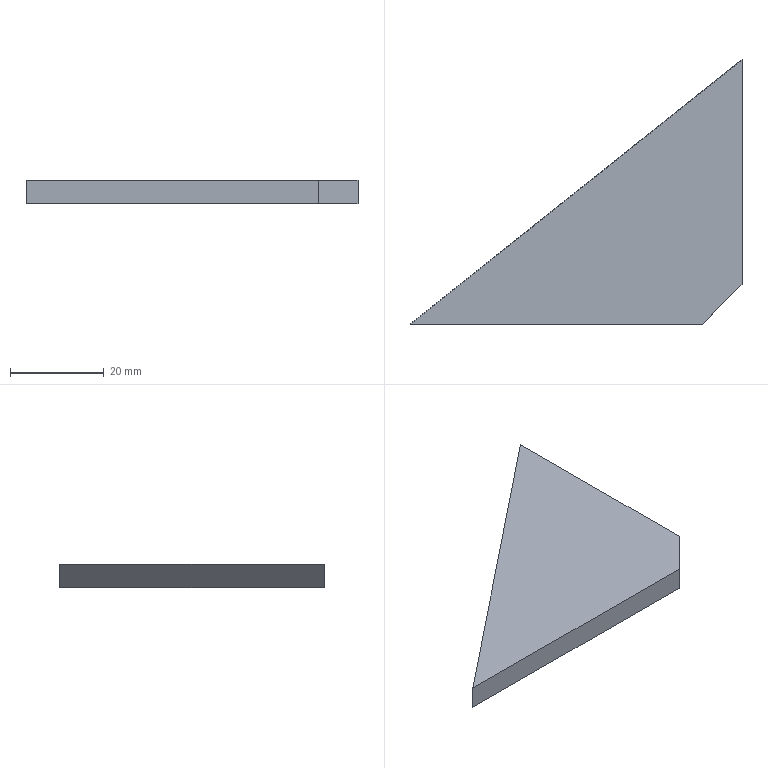Part | SolidWorks | features Extrusion 1, ICE 1 | 1 solid | 6 faces | box 70.878 x 56.464 x 5 mm | volume 9823 mm3 | plane 6
STEP:
#1=CARTESIAN_POINT('',(-5.,0.,0.));
#2=VERTEX_POINT('',#1);
#3=CARTESIAN_POINT('',(-75.878,-56.464,0.));
#4=VERTEX_POINT('',#3);
#5=CARTESIAN_POINT('',(-113.536,-86.464,0.));
#6=DIRECTION('',(-0.7821,-0.6231,0.));
#7=VECTOR('',#6,1000.);
#8=LINE('',#5,#7);
#9=EDGE_CURVE('',#2,#4,#8,.T.);
#10=ORIENTED_EDGE('',*,*,#9,.T.);
#11=CARTESIAN_POINT('',(-75.878,-56.464,5.));
#12=VERTEX_POINT('',#11);
#13=CARTESIAN_POINT('',(-75.878,-56.464,5.));
#14=DIRECTION('',(0.,0.,1.));
#15=VECTOR('',#14,1000.);
#16=LINE('',#13,#15);
#17=EDGE_CURVE('',#4,#12,#16,.T.);
#18=ORIENTED_EDGE('',*,*,#17,.T.);
#19=CARTESIAN_POINT('',(-5.,0.,5.));
#20=VERTEX_POINT('',#19);
#21=CARTESIAN_POINT('',(-113.536,-86.464,5.));
#22=DIRECTION('',(-0.7821,-0.6231,0.));
#23=VECTOR('',#22,1000.);
#24=LINE('',#21,#23);
#25=EDGE_CURVE('',#20,#12,#24,.T.);
#26=ORIENTED_EDGE('',*,*,#25,.F.);
#27=CARTESIAN_POINT('',(-5.,0.,5.));
#28=DIRECTION('',(0.,0.,-1.));
#29=VECTOR('',#28,1000.);
#30=LINE('',#27,#29);
#31=EDGE_CURVE('',#20,#2,#30,.T.);
#32=ORIENTED_EDGE('',*,*,#31,.T.);
#33=EDGE_LOOP('',(#10,#18,#26,#32));
#34=FACE_OUTER_BOUND('',#33,.T.);
#35=CARTESIAN_POINT('',(-113.536,-86.464,5.));
#36=DIRECTION('',(0.6231,-0.7821,0.));
#37=DIRECTION('',(0.7821,0.6231,0.));
#38=AXIS2_PLACEMENT_3D('',#35,#36,#37);
#39=PLANE('',#38);
#40=ADVANCED_FACE('',(#34),#39,.F.);
#41=CARTESIAN_POINT('',(-13.536,-56.464,5.));
#42=VERTEX_POINT('',#41);
#43=CARTESIAN_POINT('',(-5.,-47.929,5.));
#44=VERTEX_POINT('',#43);
#45=CARTESIAN_POINT('',(-5.,-47.929,5.));
#46=DIRECTION('',(0.7071,0.7071,0.));
#47=VECTOR('',#46,1000.);
#48=LINE('',#45,#47);
#49=EDGE_CURVE('',#42,#44,#48,.T.);
#50=ORIENTED_EDGE('',*,*,#49,.F.);
#51=CARTESIAN_POINT('',(-13.536,-56.464,0.));
#52=VERTEX_POINT('',#51);
#53=CARTESIAN_POINT('',(-13.536,-56.464,-355.));
#54=DIRECTION('',(0.,0.,1.));
#55=VECTOR('',#54,1000.);
#56=LINE('',#53,#55);
#57=EDGE_CURVE('',#52,#42,#56,.T.);
#58=ORIENTED_EDGE('',*,*,#57,.F.);
#59=CARTESIAN_POINT('',(-5.,-47.929,0.));
#60=VERTEX_POINT('',#59);
#61=CARTESIAN_POINT('',(-5.,-47.929,0.));
#62=DIRECTION('',(0.7071,0.7071,0.));
#63=VECTOR('',#62,1000.);
#64=LINE('',#61,#63);
#65=EDGE_CURVE('',#52,#60,#64,.T.);
#66=ORIENTED_EDGE('',*,*,#65,.T.);
#67=CARTESIAN_POINT('',(-5.,-47.929,5.));
#68=DIRECTION('',(0.,0.,-1.));
#69=VECTOR('',#68,1000.);
#70=LINE('',#67,#69);
#71=EDGE_CURVE('',#44,#60,#70,.T.);
#72=ORIENTED_EDGE('',*,*,#71,.F.);
#73=EDGE_LOOP('',(#50,#58,#66,#72));
#74=FACE_OUTER_BOUND('',#73,.T.);
#75=CARTESIAN_POINT('',(-5.,-47.929,5.));
#76=DIRECTION('',(-0.7071,0.7071,0.));
#77=DIRECTION('',(-0.7071,-0.7071,0.));
#78=AXIS2_PLACEMENT_3D('',#75,#76,#77);
#79=PLANE('',#78);
#80=ADVANCED_FACE('',(#74),#79,.F.);
#81=CARTESIAN_POINT('',(-5.,0.,0.));
#82=DIRECTION('',(0.,1.,0.));
#83=VECTOR('',#82,1000.);
#84=LINE('',#81,#83);
#85=EDGE_CURVE('',#60,#2,#84,.T.);
#86=ORIENTED_EDGE('',*,*,#85,.T.);
#87=ORIENTED_EDGE('',*,*,#31,.F.);
#88=CARTESIAN_POINT('',(-5.,0.,5.));
#89=DIRECTION('',(0.,1.,0.));
#90=VECTOR('',#89,1000.);
#91=LINE('',#88,#90);
#92=EDGE_CURVE('',#44,#20,#91,.T.);
#93=ORIENTED_EDGE('',*,*,#92,.F.);
#94=ORIENTED_EDGE('',*,*,#71,.T.);
#95=EDGE_LOOP('',(#86,#87,#93,#94));
#96=FACE_OUTER_BOUND('',#95,.T.);
#97=CARTESIAN_POINT('',(-5.,0.,5.));
#98=DIRECTION('',(-1.,0.,0.));
#99=DIRECTION('',(0.,0.,1.));
#100=AXIS2_PLACEMENT_3D('',#97,#98,#99);
#101=PLANE('',#100);
#102=ADVANCED_FACE('',(#96),#101,.F.);
#103=ORIENTED_EDGE('',*,*,#25,.T.);
#104=CARTESIAN_POINT('',(-113.536,-56.464,5.));
#105=DIRECTION('',(-1.,0.,0.));
#106=VECTOR('',#105,1000.);
#107=LINE('',#104,#106);
#108=EDGE_CURVE('',#42,#12,#107,.T.);
#109=ORIENTED_EDGE('',*,*,#108,.F.);
#110=ORIENTED_EDGE('',*,*,#49,.T.);
#111=ORIENTED_EDGE('',*,*,#92,.T.);
#112=EDGE_LOOP('',(#103,#109,#110,#111));
#113=FACE_OUTER_BOUND('',#112,.T.);
#114=CARTESIAN_POINT('',(0.,0.,5.));
#115=DIRECTION('',(0.,0.,-1.));
#116=DIRECTION('',(-1.,0.,0.));
#117=AXIS2_PLACEMENT_3D('',#114,#115,#116);
#118=PLANE('',#117);
#119=ADVANCED_FACE('',(#113),#118,.F.);
#120=CARTESIAN_POINT('',(0.,-56.464,0.));
#121=DIRECTION('',(1.,0.,0.));
#122=VECTOR('',#121,1000.);
#123=LINE('',#120,#122);
#124=EDGE_CURVE('',#4,#52,#123,.T.);
#125=ORIENTED_EDGE('',*,*,#124,.F.);
#126=ORIENTED_EDGE('',*,*,#9,.F.);
#127=ORIENTED_EDGE('',*,*,#85,.F.);
#128=ORIENTED_EDGE('',*,*,#65,.F.);
#129=EDGE_LOOP('',(#125,#126,#127,#128));
#130=FACE_OUTER_BOUND('',#129,.T.);
#131=CARTESIAN_POINT('',(0.,0.,0.));
#132=DIRECTION('',(0.,0.,-1.));
#133=DIRECTION('',(-1.,0.,0.));
#134=AXIS2_PLACEMENT_3D('',#131,#132,#133);
#135=PLANE('',#134);
#136=ADVANCED_FACE('',(#130),#135,.T.);
#137=ORIENTED_EDGE('',*,*,#124,.T.);
#138=ORIENTED_EDGE('',*,*,#57,.T.);
#139=ORIENTED_EDGE('',*,*,#108,.T.);
#140=ORIENTED_EDGE('',*,*,#17,.F.);
#141=EDGE_LOOP('',(#137,#138,#139,#140));
#142=FACE_OUTER_BOUND('',#141,.T.);
#143=CARTESIAN_POINT('',(-113.536,-56.464,-355.));
#144=DIRECTION('',(0.,1.,0.));
#145=DIRECTION('',(0.,0.,1.));
#146=AXIS2_PLACEMENT_3D('',#143,#144,#145);
#147=PLANE('',#146);
#148=ADVANCED_FACE('',(#142),#147,.F.);
#149=CLOSED_SHELL('',(#40,#80,#102,#119,#136,#148));
#150=MANIFOLD_SOLID_BREP('',#149);
#151=CARTESIAN_POINT('',(0.,0.,0.));
#152=DIRECTION('',(0.,0.,1.));
#153=DIRECTION('',(1.,0.,0.));
#154=AXIS2_PLACEMENT_3D('',#151,#152,#153);
#155=(LENGTH_UNIT()NAMED_UNIT(*)SI_UNIT(.MILLI.,.METRE.));
#156=UNCERTAINTY_MEASURE_WITH_UNIT(LENGTH_MEASURE(0.00001),#155,'','');
#157=(NAMED_UNIT(*)PLANE_ANGLE_UNIT()SI_UNIT($,.RADIAN.));
#158=(NAMED_UNIT(*)SI_UNIT($,.STERADIAN.)SOLID_ANGLE_UNIT());
#159=(GEOMETRIC_REPRESENTATION_CONTEXT(3)GLOBAL_UNCERTAINTY_ASSIGNED_CONTEXT((#156))GLOBAL_UNIT_ASSIGNED_CONTEXT((#155,#157,#158))REPRESENTATION_CONTEXT('',''));
#160=ADVANCED_BREP_SHAPE_REPRESENTATION('',(#150,#154),#159);